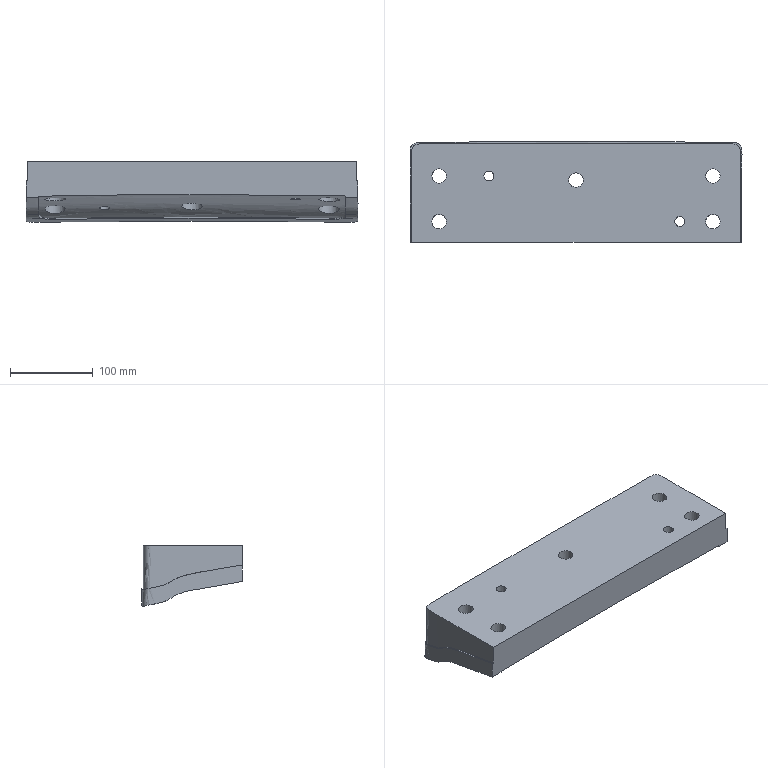Part | NX | features solid 2 | 1 solid | 36 faces | box 400.096 x 121.611 x 73.052 mm | volume 2340207 mm3 | cylinder 14 | spline 12 | plane 10 | commonest cylinder face diameters 17.5 x5 25 x5 12 x2 30 x2